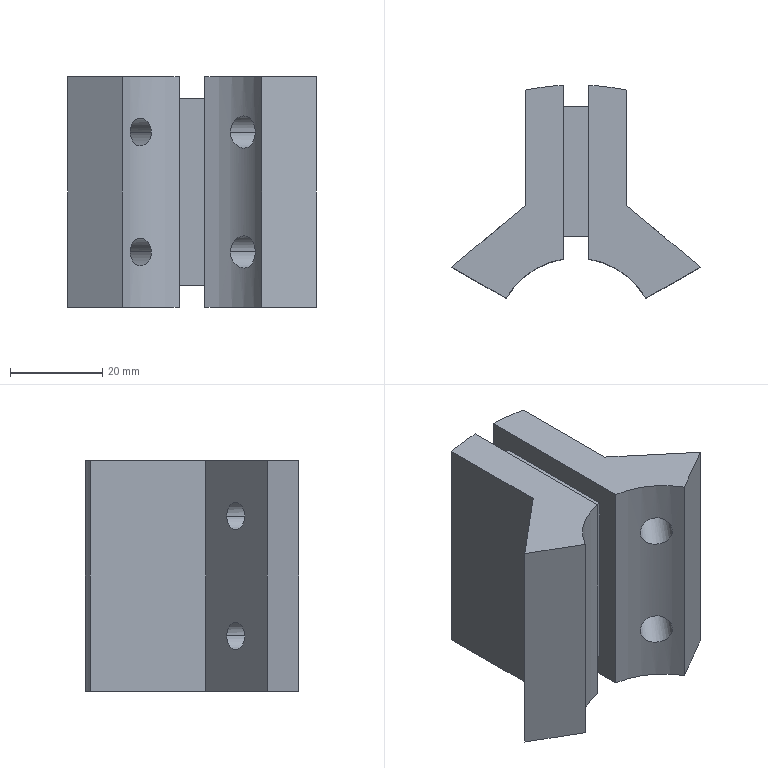Part | SolidWorks | features 3DProfileFeature 2, HoleWzd 2, Extrusion 1, ICE 1 | 1 solid | 28 faces | box 53.823 x 46.181 x 50 mm | volume 52873 mm3 | plane 16 | cylinder 12 | commonest cylinder face diameters 6 x4 7 x4 35 x2 110 x2
STEP:
#1=CARTESIAN_POINT('',(13.703,10.885,13.));
#2=VERTEX_POINT('',#1);
#3=CARTESIAN_POINT('',(8.34,15.385,13.));
#4=VERTEX_POINT('',#3);
#5=CARTESIAN_POINT('',(13.703,10.885,13.));
#6=CARTESIAN_POINT('',(13.703,10.885,12.771));
#7=CARTESIAN_POINT('',(13.689,10.903,12.544));
#8=CARTESIAN_POINT('',(13.631,10.975,12.09));
#9=CARTESIAN_POINT('',(13.588,11.028,11.87));
#10=CARTESIAN_POINT('',(13.476,11.165,11.449));
#11=CARTESIAN_POINT('',(13.405,11.251,11.245));
#12=CARTESIAN_POINT('',(13.237,11.447,10.864));
#13=CARTESIAN_POINT('',(13.141,11.558,10.688));
#14=CARTESIAN_POINT('',(12.924,11.8,10.365));
#15=CARTESIAN_POINT('',(12.801,11.934,10.218));
#16=CARTESIAN_POINT('',(12.538,12.21,9.964));
#17=CARTESIAN_POINT('',(12.397,12.353,9.856));
#18=CARTESIAN_POINT('',(12.093,12.651,9.68));
#19=CARTESIAN_POINT('',(11.932,12.804,9.613));
#20=CARTESIAN_POINT('',(11.6,13.105,9.523));
#21=CARTESIAN_POINT('',(11.427,13.256,9.5));
#22=CARTESIAN_POINT('',(11.073,13.553,9.5));
#23=CARTESIAN_POINT('',(10.896,13.696,9.522));
#24=CARTESIAN_POINT('',(10.541,13.971,9.611));
#25=CARTESIAN_POINT('',(10.362,14.104,9.679));
#26=CARTESIAN_POINT('',(10.017,14.351,9.854));
#27=CARTESIAN_POINT('',(9.85,14.466,9.962));
#28=CARTESIAN_POINT('',(9.531,14.678,10.216));
#29=CARTESIAN_POINT('',(9.379,14.775,10.363));
#30=CARTESIAN_POINT('',(8.965,15.033,10.845));
#31=CARTESIAN_POINT('',(8.735,15.165,11.234));
#32=CARTESIAN_POINT('',(8.502,15.296,11.866));
#33=CARTESIAN_POINT('',(8.442,15.329,12.088));
#34=CARTESIAN_POINT('',(8.361,15.374,12.539));
#35=CARTESIAN_POINT('',(8.34,15.385,12.768));
#36=CARTESIAN_POINT('',(8.34,15.385,13.));
#37=B_SPLINE_CURVE_WITH_KNOTS('',3,(#5,#6,#7,#8,#9,#10,#11,#12,#13,#14,#15,#16,#17,#18,#19,#20,#21,#22,#23,#24,#25,#26,#27,#28,#29,#30,#31,#32,#33,#34,#35,#36),.UNSPECIFIED.,.F.,.F.,(4,2,2,2,2,2,2,2,2,2,2,2,2,2,2,4),(0.01097,0.01166,0.01234,0.01303,0.01371,0.0144,0.01508,0.01577,0.01645,0.01714,0.01782,0.01851,0.0192,0.02057,0.02125,0.02194),.UNSPECIFIED.);
#38=EDGE_CURVE('',#2,#4,#37,.T.);
#39=ORIENTED_EDGE('',*,*,#38,.F.);
#40=CARTESIAN_POINT('',(21.451,20.119,13.));
#41=VERTEX_POINT('',#40);
#42=CARTESIAN_POINT('',(21.451,20.119,13.));
#43=DIRECTION('',(0.6428,0.766,0.));
#44=VECTOR('',#43,1000.);
#45=LINE('',#42,#44);
#46=EDGE_CURVE('',#2,#41,#45,.T.);
#47=ORIENTED_EDGE('',*,*,#46,.T.);
#48=CARTESIAN_POINT('',(16.089,24.619,13.));
#49=VERTEX_POINT('',#48);
#50=CARTESIAN_POINT('',(18.77,22.369,13.));
#51=DIRECTION('',(0.6428,0.766,0.));
#52=DIRECTION('',(-0.766,0.6428,0.));
#53=AXIS2_PLACEMENT_3D('',#50,#51,#52);
#54=CIRCLE('',#53,3.5);
#55=EDGE_CURVE('',#41,#49,#54,.T.);
#56=ORIENTED_EDGE('',*,*,#55,.T.);
#57=CARTESIAN_POINT('',(16.089,24.619,13.));
#58=DIRECTION('',(0.6428,0.766,0.));
#59=VECTOR('',#58,1000.);
#60=LINE('',#57,#59);
#61=EDGE_CURVE('',#4,#49,#60,.T.);
#62=ORIENTED_EDGE('',*,*,#61,.F.);
#63=EDGE_LOOP('',(#39,#47,#56,#62));
#64=FACE_OUTER_BOUND('',#63,.T.);
#65=CARTESIAN_POINT('',(18.77,22.369,13.));
#66=DIRECTION('',(0.6428,0.766,0.));
#67=DIRECTION('',(-0.766,0.6428,0.));
#68=AXIS2_PLACEMENT_3D('',#65,#66,#67);
#69=CYLINDRICAL_SURFACE('',#68,3.5);
#70=ADVANCED_FACE('',(#64),#69,.F.);
#71=CARTESIAN_POINT('',(13.703,10.885,-13.));
#72=VERTEX_POINT('',#71);
#73=CARTESIAN_POINT('',(8.34,15.385,-13.));
#74=VERTEX_POINT('',#73);
#75=CARTESIAN_POINT('',(13.703,10.885,-13.));
#76=CARTESIAN_POINT('',(13.703,10.885,-13.229));
#77=CARTESIAN_POINT('',(13.689,10.903,-13.456));
#78=CARTESIAN_POINT('',(13.631,10.975,-13.91));
#79=CARTESIAN_POINT('',(13.588,11.028,-14.13));
#80=CARTESIAN_POINT('',(13.476,11.165,-14.551));
#81=CARTESIAN_POINT('',(13.405,11.251,-14.755));
#82=CARTESIAN_POINT('',(13.237,11.447,-15.136));
#83=CARTESIAN_POINT('',(13.141,11.558,-15.312));
#84=CARTESIAN_POINT('',(12.924,11.8,-15.635));
#85=CARTESIAN_POINT('',(12.801,11.934,-15.782));
#86=CARTESIAN_POINT('',(12.538,12.21,-16.036));
#87=CARTESIAN_POINT('',(12.397,12.353,-16.144));
#88=CARTESIAN_POINT('',(12.093,12.651,-16.32));
#89=CARTESIAN_POINT('',(11.932,12.804,-16.387));
#90=CARTESIAN_POINT('',(11.6,13.105,-16.477));
#91=CARTESIAN_POINT('',(11.427,13.256,-16.5));
#92=CARTESIAN_POINT('',(11.073,13.553,-16.5));
#93=CARTESIAN_POINT('',(10.896,13.696,-16.478));
#94=CARTESIAN_POINT('',(10.541,13.971,-16.389));
#95=CARTESIAN_POINT('',(10.362,14.104,-16.321));
#96=CARTESIAN_POINT('',(10.017,14.351,-16.146));
#97=CARTESIAN_POINT('',(9.85,14.466,-16.038));
#98=CARTESIAN_POINT('',(9.531,14.678,-15.784));
#99=CARTESIAN_POINT('',(9.379,14.775,-15.637));
#100=CARTESIAN_POINT('',(8.965,15.033,-15.155));
#101=CARTESIAN_POINT('',(8.735,15.165,-14.766));
#102=CARTESIAN_POINT('',(8.502,15.296,-14.134));
#103=CARTESIAN_POINT('',(8.442,15.329,-13.912));
#104=CARTESIAN_POINT('',(8.361,15.374,-13.461));
#105=CARTESIAN_POINT('',(8.34,15.385,-13.232));
#106=CARTESIAN_POINT('',(8.34,15.385,-13.));
#107=B_SPLINE_CURVE_WITH_KNOTS('',3,(#75,#76,#77,#78,#79,#80,#81,#82,#83,#84,#85,#86,#87,#88,#89,#90,#91,#92,#93,#94,#95,#96,#97,#98,#99,#100,#101,#102,#103,#104,#105,#106),.UNSPECIFIED.,.F.,.F.,(4,2,2,2,2,2,2,2,2,2,2,2,2,2,2,4),(0.01097,0.01166,0.01234,0.01303,0.01371,0.0144,0.01508,0.01577,0.01645,0.01714,0.01782,0.01851,0.0192,0.02057,0.02125,0.02194),.UNSPECIFIED.);
#108=EDGE_CURVE('',#72,#74,#107,.T.);
#109=ORIENTED_EDGE('',*,*,#108,.F.);
#110=CARTESIAN_POINT('',(21.451,20.119,-13.));
#111=VERTEX_POINT('',#110);
#112=CARTESIAN_POINT('',(21.451,20.119,-13.));
#113=DIRECTION('',(0.6428,0.766,0.));
#114=VECTOR('',#113,1000.);
#115=LINE('',#112,#114);
#116=EDGE_CURVE('',#72,#111,#115,.T.);
#117=ORIENTED_EDGE('',*,*,#116,.T.);
#118=CARTESIAN_POINT('',(16.089,24.619,-13.));
#119=VERTEX_POINT('',#118);
#120=CARTESIAN_POINT('',(18.77,22.369,-13.));
#121=DIRECTION('',(0.6428,0.766,0.));
#122=DIRECTION('',(-0.766,0.6428,0.));
#123=AXIS2_PLACEMENT_3D('',#120,#121,#122);
#124=CIRCLE('',#123,3.5);
#125=EDGE_CURVE('',#111,#119,#124,.T.);
#126=ORIENTED_EDGE('',*,*,#125,.T.);
#127=CARTESIAN_POINT('',(16.089,24.619,-13.));
#128=DIRECTION('',(0.6428,0.766,0.));
#129=VECTOR('',#128,1000.);
#130=LINE('',#127,#129);
#131=EDGE_CURVE('',#74,#119,#130,.T.);
#132=ORIENTED_EDGE('',*,*,#131,.F.);
#133=EDGE_LOOP('',(#109,#117,#126,#132));
#134=FACE_OUTER_BOUND('',#133,.T.);
#135=CARTESIAN_POINT('',(18.77,22.369,-13.));
#136=DIRECTION('',(0.6428,0.766,0.));
#137=DIRECTION('',(-0.766,0.6428,0.));
#138=AXIS2_PLACEMENT_3D('',#135,#136,#137);
#139=CYLINDRICAL_SURFACE('',#138,3.5);
#140=ADVANCED_FACE('',(#134),#139,.F.);
#141=CARTESIAN_POINT('',(-8.784,15.136,-13.));
#142=VERTEX_POINT('',#141);
#143=CARTESIAN_POINT('',(-13.38,11.279,-13.));
#144=VERTEX_POINT('',#143);
#145=CARTESIAN_POINT('',(-8.784,15.136,-13.));
#146=CARTESIAN_POINT('',(-8.784,15.136,-13.196));
#147=CARTESIAN_POINT('',(-8.801,15.126,-13.391));
#148=CARTESIAN_POINT('',(-8.868,15.087,-13.779));
#149=CARTESIAN_POINT('',(-8.919,15.057,-13.968));
#150=CARTESIAN_POINT('',(-9.049,14.979,-14.329));
#151=CARTESIAN_POINT('',(-9.13,14.93,-14.504));
#152=CARTESIAN_POINT('',(-9.317,14.814,-14.831));
#153=CARTESIAN_POINT('',(-9.423,14.747,-14.982));
#154=CARTESIAN_POINT('',(-9.656,14.595,-15.258));
#155=CARTESIAN_POINT('',(-9.785,14.509,-15.385));
#156=CARTESIAN_POINT('',(-10.054,14.324,-15.602));
#157=CARTESIAN_POINT('',(-10.195,14.225,-15.695));
#158=CARTESIAN_POINT('',(-10.489,14.009,-15.846));
#159=CARTESIAN_POINT('',(-10.641,13.894,-15.904));
#160=CARTESIAN_POINT('',(-10.943,13.658,-15.98));
#161=CARTESIAN_POINT('',(-11.096,13.534,-16.));
#162=CARTESIAN_POINT('',(-11.399,13.28,-16.));
#163=CARTESIAN_POINT('',(-11.547,13.152,-15.981));
#164=CARTESIAN_POINT('',(-11.833,12.895,-15.905));
#165=CARTESIAN_POINT('',(-11.973,12.765,-15.847));
#166=CARTESIAN_POINT('',(-12.235,12.513,-15.697));
#167=CARTESIAN_POINT('',(-12.358,12.392,-15.605));
#168=CARTESIAN_POINT('',(-12.588,12.158,-15.387));
#169=CARTESIAN_POINT('',(-12.695,12.046,-15.261));
#170=CARTESIAN_POINT('',(-12.98,11.741,-14.847));
#171=CARTESIAN_POINT('',(-13.129,11.571,-14.513));
#172=CARTESIAN_POINT('',(-13.279,11.399,-13.972));
#173=CARTESIAN_POINT('',(-13.317,11.354,-13.782));
#174=CARTESIAN_POINT('',(-13.368,11.294,-13.395));
#175=CARTESIAN_POINT('',(-13.38,11.279,-13.199));
#176=CARTESIAN_POINT('',(-13.38,11.279,-13.));
#177=B_SPLINE_CURVE_WITH_KNOTS('',3,(#145,#146,#147,#148,#149,#150,#151,#152,#153,#154,#155,#156,#157,#158,#159,#160,#161,#162,#163,#164,#165,#166,#167,#168,#169,#170,#171,#172,#173,#174,#175,#176),.UNSPECIFIED.,.F.,.F.,(4,2,2,2,2,2,2,2,2,2,2,2,2,2,2,4),(0.009397,0.009984,0.01057,0.01116,0.01175,0.01233,0.01292,0.01351,0.01409,0.01468,0.01527,0.01586,0.01644,0.01762,0.0182,0.01879),.UNSPECIFIED.);
#178=EDGE_CURVE('',#142,#144,#177,.T.);
#179=ORIENTED_EDGE('',*,*,#178,.F.);
#180=CARTESIAN_POINT('',(-16.472,24.297,-13.));
#181=VERTEX_POINT('',#180);
#182=CARTESIAN_POINT('',(-16.472,24.297,-13.));
#183=DIRECTION('',(-0.6428,0.766,0.));
#184=VECTOR('',#183,1000.);
#185=LINE('',#182,#184);
#186=EDGE_CURVE('',#142,#181,#185,.T.);
#187=ORIENTED_EDGE('',*,*,#186,.T.);
#188=CARTESIAN_POINT('',(-21.068,20.441,-13.));
#189=VERTEX_POINT('',#188);
#190=CARTESIAN_POINT('',(-18.77,22.369,-13.));
#191=DIRECTION('',(-0.6428,0.766,0.));
#192=DIRECTION('',(-0.766,-0.6428,0.));
#193=AXIS2_PLACEMENT_3D('',#190,#191,#192);
#194=CIRCLE('',#193,3.);
#195=EDGE_CURVE('',#181,#189,#194,.T.);
#196=ORIENTED_EDGE('',*,*,#195,.T.);
#197=CARTESIAN_POINT('',(-21.068,20.441,-13.));
#198=DIRECTION('',(-0.6428,0.766,0.));
#199=VECTOR('',#198,1000.);
#200=LINE('',#197,#199);
#201=EDGE_CURVE('',#144,#189,#200,.T.);
#202=ORIENTED_EDGE('',*,*,#201,.F.);
#203=EDGE_LOOP('',(#179,#187,#196,#202));
#204=FACE_OUTER_BOUND('',#203,.T.);
#205=CARTESIAN_POINT('',(-18.77,22.369,-13.));
#206=DIRECTION('',(-0.6428,0.766,0.));
#207=DIRECTION('',(-0.766,-0.6428,0.));
#208=AXIS2_PLACEMENT_3D('',#205,#206,#207);
#209=CYLINDRICAL_SURFACE('',#208,3.);
#210=ADVANCED_FACE('',(#204),#209,.F.);
#211=CARTESIAN_POINT('',(-8.784,15.136,13.));
#212=VERTEX_POINT('',#211);
#213=CARTESIAN_POINT('',(-13.38,11.279,13.));
#214=VERTEX_POINT('',#213);
#215=CARTESIAN_POINT('',(-8.784,15.136,13.));
#216=CARTESIAN_POINT('',(-8.784,15.136,12.804));
#217=CARTESIAN_POINT('',(-8.801,15.126,12.609));
#218=CARTESIAN_POINT('',(-8.868,15.087,12.221));
#219=CARTESIAN_POINT('',(-8.919,15.057,12.032));
#220=CARTESIAN_POINT('',(-9.049,14.979,11.671));
#221=CARTESIAN_POINT('',(-9.13,14.93,11.496));
#222=CARTESIAN_POINT('',(-9.317,14.814,11.169));
#223=CARTESIAN_POINT('',(-9.423,14.747,11.018));
#224=CARTESIAN_POINT('',(-9.656,14.595,10.742));
#225=CARTESIAN_POINT('',(-9.785,14.509,10.615));
#226=CARTESIAN_POINT('',(-10.054,14.324,10.398));
#227=CARTESIAN_POINT('',(-10.195,14.225,10.305));
#228=CARTESIAN_POINT('',(-10.489,14.009,10.154));
#229=CARTESIAN_POINT('',(-10.641,13.894,10.096));
#230=CARTESIAN_POINT('',(-10.943,13.658,10.02));
#231=CARTESIAN_POINT('',(-11.096,13.534,10.));
#232=CARTESIAN_POINT('',(-11.399,13.28,10.));
#233=CARTESIAN_POINT('',(-11.547,13.152,10.019));
#234=CARTESIAN_POINT('',(-11.833,12.895,10.095));
#235=CARTESIAN_POINT('',(-11.973,12.765,10.153));
#236=CARTESIAN_POINT('',(-12.235,12.513,10.303));
#237=CARTESIAN_POINT('',(-12.358,12.392,10.395));
#238=CARTESIAN_POINT('',(-12.588,12.158,10.613));
#239=CARTESIAN_POINT('',(-12.695,12.046,10.739));
#240=CARTESIAN_POINT('',(-12.98,11.741,11.153));
#241=CARTESIAN_POINT('',(-13.129,11.571,11.487));
#242=CARTESIAN_POINT('',(-13.279,11.399,12.028));
#243=CARTESIAN_POINT('',(-13.317,11.354,12.218));
#244=CARTESIAN_POINT('',(-13.368,11.294,12.605));
#245=CARTESIAN_POINT('',(-13.38,11.279,12.801));
#246=CARTESIAN_POINT('',(-13.38,11.279,13.));
#247=B_SPLINE_CURVE_WITH_KNOTS('',3,(#215,#216,#217,#218,#219,#220,#221,#222,#223,#224,#225,#226,#227,#228,#229,#230,#231,#232,#233,#234,#235,#236,#237,#238,#239,#240,#241,#242,#243,#244,#245,#246),.UNSPECIFIED.,.F.,.F.,(4,2,2,2,2,2,2,2,2,2,2,2,2,2,2,4),(0.009397,0.009984,0.01057,0.01116,0.01175,0.01233,0.01292,0.01351,0.01409,0.01468,0.01527,0.01586,0.01644,0.01762,0.0182,0.01879),.UNSPECIFIED.);
#248=EDGE_CURVE('',#212,#214,#247,.T.);
#249=ORIENTED_EDGE('',*,*,#248,.F.);
#250=CARTESIAN_POINT('',(-16.472,24.297,13.));
#251=VERTEX_POINT('',#250);
#252=CARTESIAN_POINT('',(-16.472,24.297,13.));
#253=DIRECTION('',(-0.6428,0.766,0.));
#254=VECTOR('',#253,1000.);
#255=LINE('',#252,#254);
#256=EDGE_CURVE('',#212,#251,#255,.T.);
#257=ORIENTED_EDGE('',*,*,#256,.T.);
#258=CARTESIAN_POINT('',(-21.068,20.441,13.));
#259=VERTEX_POINT('',#258);
#260=CARTESIAN_POINT('',(-18.77,22.369,13.));
#261=DIRECTION('',(-0.6428,0.766,0.));
#262=DIRECTION('',(-0.766,-0.6428,0.));
#263=AXIS2_PLACEMENT_3D('',#260,#261,#262);
#264=CIRCLE('',#263,3.);
#265=EDGE_CURVE('',#251,#259,#264,.T.);
#266=ORIENTED_EDGE('',*,*,#265,.T.);
#267=CARTESIAN_POINT('',(-21.068,20.441,13.));
#268=DIRECTION('',(-0.6428,0.766,0.));
#269=VECTOR('',#268,1000.);
#270=LINE('',#267,#269);
#271=EDGE_CURVE('',#214,#259,#270,.T.);
#272=ORIENTED_EDGE('',*,*,#271,.F.);
#273=EDGE_LOOP('',(#249,#257,#266,#272));
#274=FACE_OUTER_BOUND('',#273,.T.);
#275=CARTESIAN_POINT('',(-18.77,22.369,13.));
#276=DIRECTION('',(-0.6428,0.766,0.));
#277=DIRECTION('',(-0.766,-0.6428,0.));
#278=AXIS2_PLACEMENT_3D('',#275,#276,#277);
#279=CYLINDRICAL_SURFACE('',#278,3.);
#280=ADVANCED_FACE('',(#274),#279,.F.);
#281=CARTESIAN_POINT('',(-2.75,54.931,-25.));
#282=VERTEX_POINT('',#281);
#283=CARTESIAN_POINT('',(-11.,53.889,-25.));
#284=VERTEX_POINT('',#283);
#285=CARTESIAN_POINT('',(0.,0.,-25.));
#286=DIRECTION('',(0.,0.,1.));
#287=DIRECTION('',(1.,0.,0.));
#288=AXIS2_PLACEMENT_3D('',#285,#286,#287);
#289=CIRCLE('',#288,55.);
#290=EDGE_CURVE('',#282,#284,#289,.T.);
#291=ORIENTED_EDGE('',*,*,#290,.T.);
#292=CARTESIAN_POINT('',(-11.,53.889,25.));
#293=VERTEX_POINT('',#292);
#294=CARTESIAN_POINT('',(-11.,53.889,25.));
#295=DIRECTION('',(0.,0.,-1.));
#296=VECTOR('',#295,1000.);
#297=LINE('',#294,#296);
#298=EDGE_CURVE('',#293,#284,#297,.T.);
#299=ORIENTED_EDGE('',*,*,#298,.F.);
#300=CARTESIAN_POINT('',(-2.75,54.931,25.));
#301=VERTEX_POINT('',#300);
#302=CARTESIAN_POINT('',(0.,0.,25.));
#303=DIRECTION('',(0.,0.,1.));
#304=DIRECTION('',(1.,0.,0.));
#305=AXIS2_PLACEMENT_3D('',#302,#303,#304);
#306=CIRCLE('',#305,55.);
#307=EDGE_CURVE('',#301,#293,#306,.T.);
#308=ORIENTED_EDGE('',*,*,#307,.F.);
#309=CARTESIAN_POINT('',(-2.75,54.931,25.));
#310=DIRECTION('',(0.,0.,-1.));
#311=VECTOR('',#310,1000.);
#312=LINE('',#309,#311);
#313=EDGE_CURVE('',#301,#282,#312,.T.);
#314=ORIENTED_EDGE('',*,*,#313,.T.);
#315=EDGE_LOOP('',(#291,#299,#308,#314));
#316=FACE_OUTER_BOUND('',#315,.T.);
#317=CARTESIAN_POINT('',(0.,0.,25.));
#318=DIRECTION('',(0.,0.,-1.));
#319=DIRECTION('',(-1.,0.,0.));
#320=AXIS2_PLACEMENT_3D('',#317,#318,#319);
#321=CYLINDRICAL_SURFACE('',#320,55.);
#322=ADVANCED_FACE('',(#316),#321,.T.);
#323=CARTESIAN_POINT('',(-11.,28.889,-25.));
#324=VERTEX_POINT('',#323);
#325=CARTESIAN_POINT('',(-11.,53.889,-25.));
#326=DIRECTION('',(0.,-1.,0.));
#327=VECTOR('',#326,1000.);
#328=LINE('',#325,#327);
#329=EDGE_CURVE('',#284,#324,#328,.T.);
#330=ORIENTED_EDGE('',*,*,#329,.T.);
#331=CARTESIAN_POINT('',(-11.,28.889,25.));
#332=VERTEX_POINT('',#331);
#333=CARTESIAN_POINT('',(-11.,28.889,25.));
#334=DIRECTION('',(0.,0.,-1.));
#335=VECTOR('',#334,1000.);
#336=LINE('',#333,#335);
#337=EDGE_CURVE('',#332,#324,#336,.T.);
#338=ORIENTED_EDGE('',*,*,#337,.F.);
#339=CARTESIAN_POINT('',(-11.,53.889,25.));
#340=DIRECTION('',(0.,-1.,0.));
#341=VECTOR('',#340,1000.);
#342=LINE('',#339,#341);
#343=EDGE_CURVE('',#293,#332,#342,.T.);
#344=ORIENTED_EDGE('',*,*,#343,.F.);
#345=ORIENTED_EDGE('',*,*,#298,.T.);
#346=EDGE_LOOP('',(#330,#338,#344,#345));
#347=FACE_OUTER_BOUND('',#346,.T.);
#348=CARTESIAN_POINT('',(-11.,53.889,25.));
#349=DIRECTION('',(1.,0.,0.));
#350=DIRECTION('',(0.,1.,0.));
#351=AXIS2_PLACEMENT_3D('',#348,#349,#350);
#352=PLANE('',#351);
#353=ADVANCED_FACE('',(#347),#352,.F.);
#354=CARTESIAN_POINT('',(-18.77,22.369,-13.));
#355=DIRECTION('',(-0.6428,0.766,0.));
#356=DIRECTION('',(-0.766,-0.6428,0.));
#357=AXIS2_PLACEMENT_3D('',#354,#355,#356);
#358=CIRCLE('',#357,3.);
#359=EDGE_CURVE('',#189,#181,#358,.T.);
#360=ORIENTED_EDGE('',*,*,#359,.F.);
#361=ORIENTED_EDGE('',*,*,#195,.F.);
#362=EDGE_LOOP('',(#360,#361));
#363=FACE_BOUND('',#362,.T.);
#364=CARTESIAN_POINT('',(-18.77,22.369,13.));
#365=DIRECTION('',(-0.6428,0.766,0.));
#366=DIRECTION('',(-0.766,-0.6428,0.));
#367=AXIS2_PLACEMENT_3D('',#364,#365,#366);
#368=CIRCLE('',#367,3.);
#369=EDGE_CURVE('',#259,#251,#368,.T.);
#370=ORIENTED_EDGE('',*,*,#369,.F.);
#371=ORIENTED_EDGE('',*,*,#265,.F.);
#372=EDGE_LOOP('',(#370,#371));
#373=FACE_BOUND('',#372,.T.);
#374=CARTESIAN_POINT('',(-26.912,15.537,-25.));
#375=VERTEX_POINT('',#374);
#376=CARTESIAN_POINT('',(-11.,28.889,-25.));
#377=DIRECTION('',(-0.766,-0.6428,0.));
#378=VECTOR('',#377,1000.);
#379=LINE('',#376,#378);
#380=EDGE_CURVE('',#324,#375,#379,.T.);
#381=ORIENTED_EDGE('',*,*,#380,.T.);
#382=CARTESIAN_POINT('',(-26.912,15.537,25.));
#383=VERTEX_POINT('',#382);
#384=CARTESIAN_POINT('',(-26.912,15.537,25.));
#385=DIRECTION('',(0.,0.,-1.));
#386=VECTOR('',#385,1000.);
#387=LINE('',#384,#386);
#388=EDGE_CURVE('',#383,#375,#387,.T.);
#389=ORIENTED_EDGE('',*,*,#388,.F.);
#390=CARTESIAN_POINT('',(-11.,28.889,25.));
#391=DIRECTION('',(-0.766,-0.6428,0.));
#392=VECTOR('',#391,1000.);
#393=LINE('',#390,#392);
#394=EDGE_CURVE('',#332,#383,#393,.T.);
#395=ORIENTED_EDGE('',*,*,#394,.F.);
#396=ORIENTED_EDGE('',*,*,#337,.T.);
#397=EDGE_LOOP('',(#381,#389,#395,#396));
#398=FACE_OUTER_BOUND('',#397,.T.);
#399=CARTESIAN_POINT('',(-11.,28.889,25.));
#400=DIRECTION('',(0.6428,-0.766,0.));
#401=DIRECTION('',(0.766,0.6428,0.));
#402=AXIS2_PLACEMENT_3D('',#399,#400,#401);
#403=PLANE('',#402);
#404=ADVANCED_FACE('',(#363,#373,#398),#403,.F.);
#405=CARTESIAN_POINT('',(-15.155,8.75,-25.));
#406=VERTEX_POINT('',#405);
#407=CARTESIAN_POINT('',(-26.912,15.537,-25.));
#408=DIRECTION('',(0.866,-0.5,0.));
#409=VECTOR('',#408,1000.);
#410=LINE('',#407,#409);
#411=EDGE_CURVE('',#375,#406,#410,.T.);
#412=ORIENTED_EDGE('',*,*,#411,.T.);
#413=CARTESIAN_POINT('',(-15.155,8.75,25.));
#414=VERTEX_POINT('',#413);
#415=CARTESIAN_POINT('',(-15.155,8.75,25.));
#416=DIRECTION('',(0.,0.,-1.));
#417=VECTOR('',#416,1000.);
#418=LINE('',#415,#417);
#419=EDGE_CURVE('',#414,#406,#418,.T.);
#420=ORIENTED_EDGE('',*,*,#419,.F.);
#421=CARTESIAN_POINT('',(-26.912,15.537,25.));
#422=DIRECTION('',(0.866,-0.5,0.));
#423=VECTOR('',#422,1000.);
#424=LINE('',#421,#423);
#425=EDGE_CURVE('',#383,#414,#424,.T.);
#426=ORIENTED_EDGE('',*,*,#425,.F.);
#427=ORIENTED_EDGE('',*,*,#388,.T.);
#428=EDGE_LOOP('',(#412,#420,#426,#427));
#429=FACE_OUTER_BOUND('',#428,.T.);
#430=CARTESIAN_POINT('',(-26.912,15.537,25.));
#431=DIRECTION('',(0.5,0.866,0.));
#432=DIRECTION('',(-0.866,0.5,0.));
#433=AXIS2_PLACEMENT_3D('',#430,#431,#432);
#434=PLANE('',#433);
#435=ADVANCED_FACE('',(#429),#434,.F.);
#436=CARTESIAN_POINT('',(-13.38,11.279,-13.));
#437=CARTESIAN_POINT('',(-13.38,11.279,-12.801));
#438=CARTESIAN_POINT('',(-13.368,11.294,-12.606));
#439=CARTESIAN_POINT('',(-13.317,11.353,-12.222));
#440=CARTESIAN_POINT('',(-13.279,11.398,-12.031));
#441=CARTESIAN_POINT('',(-13.179,11.513,-11.668));
#442=CARTESIAN_POINT('',(-13.118,11.584,-11.496));
#443=CARTESIAN_POINT('',(-12.971,11.748,-11.17));
#444=CARTESIAN_POINT('',(-12.886,11.842,-11.016));
#445=CARTESIAN_POINT('',(-12.696,12.045,-10.74));
#446=CARTESIAN_POINT('',(-12.591,12.155,-10.616));
#447=CARTESIAN_POINT('',(-12.36,12.39,-10.397));
#448=CARTESIAN_POINT('',(-12.236,12.513,-10.304));
#449=CARTESIAN_POINT('',(-11.974,12.763,-10.154));
#450=CARTESIAN_POINT('',(-11.836,12.892,-10.096));
#451=CARTESIAN_POINT('',(-11.547,13.151,-10.019));
#452=CARTESIAN_POINT('',(-11.4,13.279,-10.));
#453=CARTESIAN_POINT('',(-11.099,13.531,-10.));
#454=CARTESIAN_POINT('',(-10.945,13.657,-10.02));
#455=CARTESIAN_POINT('',(-10.641,13.894,-10.096));
#456=CARTESIAN_POINT('',(-10.492,14.007,-10.153));
#457=CARTESIAN_POINT('',(-10.198,14.223,-10.304));
#458=CARTESIAN_POINT('',(-10.055,14.324,-10.398));
#459=CARTESIAN_POINT('',(-9.786,14.509,-10.615));
#460=CARTESIAN_POINT('',(-9.659,14.594,-10.739));
#461=CARTESIAN_POINT('',(-9.423,14.747,-11.018));
#462=CARTESIAN_POINT('',(-9.317,14.814,-11.17));
#463=CARTESIAN_POINT('',(-9.131,14.93,-11.494));
#464=CARTESIAN_POINT('',(-9.049,14.979,-11.67));
#465=CARTESIAN_POINT('',(-8.919,15.057,-12.033));
#466=CARTESIAN_POINT('',(-8.869,15.086,-12.22));
#467=CARTESIAN_POINT('',(-8.801,15.126,-12.605));
#468=CARTESIAN_POINT('',(-8.784,15.136,-12.804));
#469=CARTESIAN_POINT('',(-8.784,15.136,-13.));
#470=B_SPLINE_CURVE_WITH_KNOTS('',3,(#436,#437,#438,#439,#440,#441,#442,#443,#444,#445,#446,#447,#448,#449,#450,#451,#452,#453,#454,#455,#456,#457,#458,#459,#460,#461,#462,#463,#464,#465,#466,#467,#468,#469),.UNSPECIFIED.,.F.,.F.,(4,2,2,2,2,2,2,2,2,2,2,2,2,2,2,2,4),(0.,0.0005873,0.001175,0.001762,0.002349,0.002936,0.003524,0.004111,0.004698,0.005286,0.005873,0.00646,0.007048,0.007635,0.008222,0.008809,0.009397),.UNSPECIFIED.);
#471=EDGE_CURVE('',#144,#142,#470,.T.);
#472=ORIENTED_EDGE('',*,*,#471,.T.);
#473=ORIENTED_EDGE('',*,*,#178,.T.);
#474=EDGE_LOOP('',(#472,#473));
#475=FACE_BOUND('',#474,.T.);
#476=CARTESIAN_POINT('',(-13.38,11.279,13.));
#477=CARTESIAN_POINT('',(-13.38,11.279,13.199));
#478=CARTESIAN_POINT('',(-13.368,11.294,13.394));
#479=CARTESIAN_POINT('',(-13.317,11.353,13.778));
#480=CARTESIAN_POINT('',(-13.279,11.398,13.969));
#481=CARTESIAN_POINT('',(-13.179,11.513,14.332));
#482=CARTESIAN_POINT('',(-13.118,11.584,14.504));
#483=CARTESIAN_POINT('',(-12.971,11.748,14.83));
#484=CARTESIAN_POINT('',(-12.886,11.842,14.984));
#485=CARTESIAN_POINT('',(-12.696,12.045,15.26));
#486=CARTESIAN_POINT('',(-12.591,12.155,15.384));
#487=CARTESIAN_POINT('',(-12.36,12.39,15.603));
#488=CARTESIAN_POINT('',(-12.236,12.513,15.696));
#489=CARTESIAN_POINT('',(-11.974,12.763,15.846));
#490=CARTESIAN_POINT('',(-11.836,12.892,15.904));
#491=CARTESIAN_POINT('',(-11.547,13.151,15.981));
#492=CARTESIAN_POINT('',(-11.4,13.279,16.));
#493=CARTESIAN_POINT('',(-11.099,13.531,16.));
#494=CARTESIAN_POINT('',(-10.945,13.657,15.98));
#495=CARTESIAN_POINT('',(-10.641,13.894,15.904));
#496=CARTESIAN_POINT('',(-10.492,14.007,15.847));
#497=CARTESIAN_POINT('',(-10.198,14.223,15.696));
#498=CARTESIAN_POINT('',(-10.055,14.324,15.602));
#499=CARTESIAN_POINT('',(-9.786,14.509,15.385));
#500=CARTESIAN_POINT('',(-9.659,14.594,15.261));
#501=CARTESIAN_POINT('',(-9.423,14.747,14.982));
#502=CARTESIAN_POINT('',(-9.317,14.814,14.83));
#503=CARTESIAN_POINT('',(-9.131,14.93,14.506));
#504=CARTESIAN_POINT('',(-9.049,14.979,14.33));
#505=CARTESIAN_POINT('',(-8.919,15.057,13.967));
#506=CARTESIAN_POINT('',(-8.869,15.086,13.78));
#507=CARTESIAN_POINT('',(-8.801,15.126,13.395));
#508=CARTESIAN_POINT('',(-8.784,15.136,13.196));
#509=CARTESIAN_POINT('',(-8.784,15.136,13.));
#510=B_SPLINE_CURVE_WITH_KNOTS('',3,(#476,#477,#478,#479,#480,#481,#482,#483,#484,#485,#486,#487,#488,#489,#490,#491,#492,#493,#494,#495,#496,#497,#498,#499,#500,#501,#502,#503,#504,#505,#506,#507,#508,#509),.UNSPECIFIED.,.F.,.F.,(4,2,2,2,2,2,2,2,2,2,2,2,2,2,2,2,4),(0.,0.0005873,0.001175,0.001762,0.002349,0.002936,0.003524,0.004111,0.004698,0.005286,0.005873,0.00646,0.007048,0.007635,0.008222,0.008809,0.009397),.UNSPECIFIED.);
#511=EDGE_CURVE('',#214,#212,#510,.T.);
#512=ORIENTED_EDGE('',*,*,#511,.T.);
#513=ORIENTED_EDGE('',*,*,#248,.T.);
#514=EDGE_LOOP('',(#512,#513));
#515=FACE_BOUND('',#514,.T.);
#516=CARTESIAN_POINT('',(-2.75,17.283,-25.));
#517=VERTEX_POINT('',#516);
#518=CARTESIAN_POINT('',(0.,0.,-25.));
#519=DIRECTION('',(0.,0.,-1.));
#520=DIRECTION('',(1.,0.,0.));
#521=AXIS2_PLACEMENT_3D('',#518,#519,#520);
#522=CIRCLE('',#521,17.5);
#523=EDGE_CURVE('',#406,#517,#522,.T.);
#524=ORIENTED_EDGE('',*,*,#523,.T.);
#525=CARTESIAN_POINT('',(-2.75,17.283,25.));
#526=VERTEX_POINT('',#525);
#527=CARTESIAN_POINT('',(-2.75,17.283,25.));
#528=DIRECTION('',(0.,0.,-1.));
#529=VECTOR('',#528,1000.);
#530=LINE('',#527,#529);
#531=EDGE_CURVE('',#526,#517,#530,.T.);
#532=ORIENTED_EDGE('',*,*,#531,.F.);
#533=CARTESIAN_POINT('',(0.,0.,25.));
#534=DIRECTION('',(0.,0.,-1.));
#535=DIRECTION('',(1.,0.,0.));
#536=AXIS2_PLACEMENT_3D('',#533,#534,#535);
#537=CIRCLE('',#536,17.5);
#538=EDGE_CURVE('',#414,#526,#537,.T.);
#539=ORIENTED_EDGE('',*,*,#538,.F.);
#540=ORIENTED_EDGE('',*,*,#419,.T.);
#541=EDGE_LOOP('',(#524,#532,#539,#540));
#542=FACE_OUTER_BOUND('',#541,.T.);
#543=CARTESIAN_POINT('',(0.,0.,25.));
#544=DIRECTION('',(0.,0.,-1.));
#545=DIRECTION('',(-1.,0.,0.));
#546=AXIS2_PLACEMENT_3D('',#543,#544,#545);
#547=CYLINDRICAL_SURFACE('',#546,17.5);
#548=ADVANCED_FACE('',(#475,#515,#542),#547,.F.);
#549=CARTESIAN_POINT('',(-2.75,50.3,20.3));
#550=VERTEX_POINT('',#549);
#551=CARTESIAN_POINT('',(-2.75,50.3,-20.3));
#552=VERTEX_POINT('',#551);
#553=CARTESIAN_POINT('',(-2.75,50.3,20.3));
#554=DIRECTION('',(0.,0.,-1.));
#555=VECTOR('',#554,1000.);
#556=LINE('',#553,#555);
#557=EDGE_CURVE('',#550,#552,#556,.T.);
#558=ORIENTED_EDGE('',*,*,#557,.T.);
#559=CARTESIAN_POINT('',(-2.75,22.2,-20.3));
#560=VERTEX_POINT('',#559);
#561=CARTESIAN_POINT('',(-2.75,22.2,-20.3));
#562=DIRECTION('',(0.,-1.,0.));
#563=VECTOR('',#562,1000.);
#564=LINE('',#561,#563);
#565=EDGE_CURVE('',#552,#560,#564,.T.);
#566=ORIENTED_EDGE('',*,*,#565,.T.);
#567=CARTESIAN_POINT('',(-2.75,22.2,20.3));
#568=VERTEX_POINT('',#567);
#569=CARTESIAN_POINT('',(-2.75,22.2,20.3));
#570=DIRECTION('',(0.,0.,-1.));
#571=VECTOR('',#570,1000.);
#572=LINE('',#569,#571);
#573=EDGE_CURVE('',#568,#560,#572,.T.);
#574=ORIENTED_EDGE('',*,*,#573,.F.);
#575=CARTESIAN_POINT('',(-2.75,22.2,20.3));
#576=DIRECTION('',(0.,-1.,0.));
#577=VECTOR('',#576,1000.);
#578=LINE('',#575,#577);
#579=EDGE_CURVE('',#550,#568,#578,.T.);
#580=ORIENTED_EDGE('',*,*,#579,.F.);
#581=EDGE_LOOP('',(#558,#566,#574,#580));
#582=FACE_BOUND('',#581,.T.);
#583=CARTESIAN_POINT('',(-2.75,54.931,-25.));
#584=DIRECTION('',(0.,1.,0.));
#585=VECTOR('',#584,1000.);
#586=LINE('',#583,#585);
#587=EDGE_CURVE('',#517,#282,#586,.T.);
#588=ORIENTED_EDGE('',*,*,#587,.T.);
#589=ORIENTED_EDGE('',*,*,#313,.F.);
#590=CARTESIAN_POINT('',(-2.75,54.931,25.));
#591=DIRECTION('',(0.,1.,0.));
#592=VECTOR('',#591,1000.);
#593=LINE('',#590,#592);
#594=EDGE_CURVE('',#526,#301,#593,.T.);
#595=ORIENTED_EDGE('',*,*,#594,.F.);
#596=ORIENTED_EDGE('',*,*,#531,.T.);
#597=EDGE_LOOP('',(#588,#589,#595,#596));
#598=FACE_OUTER_BOUND('',#597,.T.);
#599=CARTESIAN_POINT('',(-2.75,54.931,25.));
#600=DIRECTION('',(-1.,0.,0.));
#601=DIRECTION('',(0.,-1.,0.));
#602=AXIS2_PLACEMENT_3D('',#599,#600,#601);
#603=PLANE('',#602);
#604=ADVANCED_FACE('',(#582,#598),#603,.F.);
#605=ORIENTED_EDGE('',*,*,#307,.T.);
#606=ORIENTED_EDGE('',*,*,#343,.T.);
#607=ORIENTED_EDGE('',*,*,#394,.T.);
#608=ORIENTED_EDGE('',*,*,#425,.T.);
#609=ORIENTED_EDGE('',*,*,#538,.T.);
#610=ORIENTED_EDGE('',*,*,#594,.T.);
#611=EDGE_LOOP('',(#605,#606,#607,#608,#609,#610));
#612=FACE_OUTER_BOUND('',#611,.T.);
#613=CARTESIAN_POINT('',(0.,0.,25.));
#614=DIRECTION('',(0.,0.,1.));
#615=DIRECTION('',(1.,0.,0.));
#616=AXIS2_PLACEMENT_3D('',#613,#614,#615);
#617=PLANE('',#616);
#618=ADVANCED_FACE('',(#612),#617,.T.);
#619=ORIENTED_EDGE('',*,*,#290,.F.);
#620=ORIENTED_EDGE('',*,*,#587,.F.);
#621=ORIENTED_EDGE('',*,*,#523,.F.);
#622=ORIENTED_EDGE('',*,*,#411,.F.);
#623=ORIENTED_EDGE('',*,*,#380,.F.);
#624=ORIENTED_EDGE('',*,*,#329,.F.);
#625=EDGE_LOOP('',(#619,#620,#621,#622,#623,#624));
#626=FACE_OUTER_BOUND('',#625,.T.);
#627=CARTESIAN_POINT('',(0.,0.,-25.));
#628=DIRECTION('',(0.,0.,1.));
#629=DIRECTION('',(1.,0.,0.));
#630=AXIS2_PLACEMENT_3D('',#627,#628,#629);
#631=PLANE('',#630);
#632=ADVANCED_FACE('',(#626),#631,.F.);
#633=CARTESIAN_POINT('',(2.75,22.2,-20.3));
#634=VERTEX_POINT('',#633);
#635=CARTESIAN_POINT('',(2.75,22.2,-20.3));
#636=DIRECTION('',(1.,0.,0.));
#637=VECTOR('',#636,1000.);
#638=LINE('',#635,#637);
#639=EDGE_CURVE('',#560,#634,#638,.T.);
#640=ORIENTED_EDGE('',*,*,#639,.T.);
#641=CARTESIAN_POINT('',(2.75,22.2,20.3));
#642=VERTEX_POINT('',#641);
#643=CARTESIAN_POINT('',(2.75,22.2,20.3));
#644=DIRECTION('',(0.,0.,-1.));
#645=VECTOR('',#644,1000.);
#646=LINE('',#643,#645);
#647=EDGE_CURVE('',#642,#634,#646,.T.);
#648=ORIENTED_EDGE('',*,*,#647,.F.);
#649=CARTESIAN_POINT('',(2.75,22.2,20.3));
#650=DIRECTION('',(1.,0.,0.));
#651=VECTOR('',#650,1000.);
#652=LINE('',#649,#651);
#653=EDGE_CURVE('',#568,#642,#652,.T.);
#654=ORIENTED_EDGE('',*,*,#653,.F.);
#655=ORIENTED_EDGE('',*,*,#573,.T.);
#656=EDGE_LOOP('',(#640,#648,#654,#655));
#657=FACE_OUTER_BOUND('',#656,.T.);
#658=CARTESIAN_POINT('',(2.75,22.2,20.3));
#659=DIRECTION('',(0.,1.,0.));
#660=DIRECTION('',(0.,0.,1.));
#661=AXIS2_PLACEMENT_3D('',#658,#659,#660);
#662=PLANE('',#661);
#663=ADVANCED_FACE('',(#657),#662,.F.);
#664=CARTESIAN_POINT('',(2.75,50.3,-20.3));
#665=VERTEX_POINT('',#664);
#666=CARTESIAN_POINT('',(2.75,50.3,-20.3));
#667=DIRECTION('',(-1.,0.,0.));
#668=VECTOR('',#667,1000.);
#669=LINE('',#666,#668);
#670=EDGE_CURVE('',#665,#552,#669,.T.);
#671=ORIENTED_EDGE('',*,*,#670,.T.);
#672=ORIENTED_EDGE('',*,*,#557,.F.);
#673=CARTESIAN_POINT('',(2.75,50.3,20.3));
#674=VERTEX_POINT('',#673);
#675=CARTESIAN_POINT('',(2.75,50.3,20.3));
#676=DIRECTION('',(-1.,0.,0.));
#677=VECTOR('',#676,1000.);
#678=LINE('',#675,#677);
#679=EDGE_CURVE('',#674,#550,#678,.T.);
#680=ORIENTED_EDGE('',*,*,#679,.F.);
#681=CARTESIAN_POINT('',(2.75,50.3,20.3));
#682=DIRECTION('',(0.,0.,-1.));
#683=VECTOR('',#682,1000.);
#684=LINE('',#681,#683);
#685=EDGE_CURVE('',#674,#665,#684,.T.);
#686=ORIENTED_EDGE('',*,*,#685,.T.);
#687=EDGE_LOOP('',(#671,#672,#680,#686));
#688=FACE_OUTER_BOUND('',#687,.T.);
#689=CARTESIAN_POINT('',(2.75,50.3,20.3));
#690=DIRECTION('',(0.,-1.,0.));
#691=DIRECTION('',(0.,0.,-1.));
#692=AXIS2_PLACEMENT_3D('',#689,#690,#691);
#693=PLANE('',#692);
#694=ADVANCED_FACE('',(#688),#693,.F.);
#695=ORIENTED_EDGE('',*,*,#579,.T.);
#696=ORIENTED_EDGE('',*,*,#653,.T.);
#697=CARTESIAN_POINT('',(2.75,22.2,20.3));
#698=DIRECTION('',(0.,1.,0.));
#699=VECTOR('',#698,1000.);
#700=LINE('',#697,#699);
#701=EDGE_CURVE('',#642,#674,#700,.T.);
#702=ORIENTED_EDGE('',*,*,#701,.T.);
#703=ORIENTED_EDGE('',*,*,#679,.T.);
#704=EDGE_LOOP('',(#695,#696,#702,#703));
#705=FACE_OUTER_BOUND('',#704,.T.);
#706=CARTESIAN_POINT('',(0.,0.,20.3));
#707=DIRECTION('',(0.,0.,1.));
#708=DIRECTION('',(1.,0.,0.));
#709=AXIS2_PLACEMENT_3D('',#706,#707,#708);
#710=PLANE('',#709);
#711=ADVANCED_FACE('',(#705),#710,.T.);
#712=ORIENTED_EDGE('',*,*,#565,.F.);
#713=ORIENTED_EDGE('',*,*,#670,.F.);
#714=CARTESIAN_POINT('',(2.75,22.2,-20.3));
#715=DIRECTION('',(0.,1.,0.));
#716=VECTOR('',#715,1000.);
#717=LINE('',#714,#716);
#718=EDGE_CURVE('',#634,#665,#717,.T.);
#719=ORIENTED_EDGE('',*,*,#718,.F.);
#720=ORIENTED_EDGE('',*,*,#639,.F.);
#721=EDGE_LOOP('',(#712,#713,#719,#720));
#722=FACE_OUTER_BOUND('',#721,.T.);
#723=CARTESIAN_POINT('',(0.,0.,-20.3));
#724=DIRECTION('',(0.,0.,1.));
#725=DIRECTION('',(1.,0.,0.));
#726=AXIS2_PLACEMENT_3D('',#723,#724,#725);
#727=PLANE('',#726);
#728=ADVANCED_FACE('',(#722),#727,.F.);
#729=CARTESIAN_POINT('',(2.75,54.931,-25.));
#730=VERTEX_POINT('',#729);
#731=CARTESIAN_POINT('',(2.75,17.283,-25.));
#732=VERTEX_POINT('',#731);
#733=CARTESIAN_POINT('',(2.75,54.931,-25.));
#734=DIRECTION('',(0.,-1.,0.));
#735=VECTOR('',#734,1000.);
#736=LINE('',#733,#735);
#737=EDGE_CURVE('',#730,#732,#736,.T.);
#738=ORIENTED_EDGE('',*,*,#737,.T.);
#739=CARTESIAN_POINT('',(2.75,17.283,25.));
#740=VERTEX_POINT('',#739);
#741=CARTESIAN_POINT('',(2.75,17.283,25.));
#742=DIRECTION('',(0.,0.,-1.));
#743=VECTOR('',#742,1000.);
#744=LINE('',#741,#743);
#745=EDGE_CURVE('',#740,#732,#744,.T.);
#746=ORIENTED_EDGE('',*,*,#745,.F.);
#747=CARTESIAN_POINT('',(2.75,54.931,25.));
#748=VERTEX_POINT('',#747);
#749=CARTESIAN_POINT('',(2.75,54.931,25.));
#750=DIRECTION('',(0.,-1.,0.));
#751=VECTOR('',#750,1000.);
#752=LINE('',#749,#751);
#753=EDGE_CURVE('',#748,#740,#752,.T.);
#754=ORIENTED_EDGE('',*,*,#753,.F.);
#755=CARTESIAN_POINT('',(2.75,54.931,25.));
#756=DIRECTION('',(0.,0.,-1.));
#757=VECTOR('',#756,1000.);
#758=LINE('',#755,#757);
#759=EDGE_CURVE('',#748,#730,#758,.T.);
#760=ORIENTED_EDGE('',*,*,#759,.T.);
#761=EDGE_LOOP('',(#738,#746,#754,#760));
#762=FACE_OUTER_BOUND('',#761,.T.);
#763=ORIENTED_EDGE('',*,*,#647,.T.);
#764=ORIENTED_EDGE('',*,*,#718,.T.);
#765=ORIENTED_EDGE('',*,*,#685,.F.);
#766=ORIENTED_EDGE('',*,*,#701,.F.);
#767=EDGE_LOOP('',(#763,#764,#765,#766));
#768=FACE_BOUND('',#767,.T.);
#769=CARTESIAN_POINT('',(2.75,54.931,25.));
#770=DIRECTION('',(1.,0.,0.));
#771=DIRECTION('',(0.,1.,0.));
#772=AXIS2_PLACEMENT_3D('',#769,#770,#771);
#773=PLANE('',#772);
#774=ADVANCED_FACE('',(#762,#768),#773,.F.);
#775=CARTESIAN_POINT('',(11.,28.889,-25.));
#776=VERTEX_POINT('',#775);
#777=CARTESIAN_POINT('',(11.,53.889,-25.));
#778=VERTEX_POINT('',#777);
#779=CARTESIAN_POINT('',(11.,53.889,-25.));
#780=DIRECTION('',(0.,1.,0.));
#781=VECTOR('',#780,1000.);
#782=LINE('',#779,#781);
#783=EDGE_CURVE('',#776,#778,#782,.T.);
#784=ORIENTED_EDGE('',*,*,#783,.T.);
#785=CARTESIAN_POINT('',(11.,53.889,25.));
#786=VERTEX_POINT('',#785);
#787=CARTESIAN_POINT('',(11.,53.889,25.));
#788=DIRECTION('',(0.,0.,-1.));
#789=VECTOR('',#788,1000.);
#790=LINE('',#787,#789);
#791=EDGE_CURVE('',#786,#778,#790,.T.);
#792=ORIENTED_EDGE('',*,*,#791,.F.);
#793=CARTESIAN_POINT('',(11.,28.889,25.));
#794=VERTEX_POINT('',#793);
#795=CARTESIAN_POINT('',(11.,53.889,25.));
#796=DIRECTION('',(0.,1.,0.));
#797=VECTOR('',#796,1000.);
#798=LINE('',#795,#797);
#799=EDGE_CURVE('',#794,#786,#798,.T.);
#800=ORIENTED_EDGE('',*,*,#799,.F.);
#801=CARTESIAN_POINT('',(11.,28.889,25.));
#802=DIRECTION('',(0.,0.,-1.));
#803=VECTOR('',#802,1000.);
#804=LINE('',#801,#803);
#805=EDGE_CURVE('',#794,#776,#804,.T.);
#806=ORIENTED_EDGE('',*,*,#805,.T.);
#807=EDGE_LOOP('',(#784,#792,#800,#806));
#808=FACE_OUTER_BOUND('',#807,.T.);
#809=CARTESIAN_POINT('',(11.,53.889,25.));
#810=DIRECTION('',(-1.,0.,0.));
#811=DIRECTION('',(0.,-1.,0.));
#812=AXIS2_PLACEMENT_3D('',#809,#810,#811);
#813=PLANE('',#812);
#814=ADVANCED_FACE('',(#808),#813,.F.);
#815=CARTESIAN_POINT('',(0.,0.,-25.));
#816=DIRECTION('',(0.,0.,1.));
#817=DIRECTION('',(1.,0.,0.));
#818=AXIS2_PLACEMENT_3D('',#815,#816,#817);
#819=CIRCLE('',#818,55.);
#820=EDGE_CURVE('',#778,#730,#819,.T.);
#821=ORIENTED_EDGE('',*,*,#820,.T.);
#822=ORIENTED_EDGE('',*,*,#759,.F.);
#823=CARTESIAN_POINT('',(0.,0.,25.));
#824=DIRECTION('',(0.,0.,1.));
#825=DIRECTION('',(1.,0.,0.));
#826=AXIS2_PLACEMENT_3D('',#823,#824,#825);
#827=CIRCLE('',#826,55.);
#828=EDGE_CURVE('',#786,#748,#827,.T.);
#829=ORIENTED_EDGE('',*,*,#828,.F.);
#830=ORIENTED_EDGE('',*,*,#791,.T.);
#831=EDGE_LOOP('',(#821,#822,#829,#830));
#832=FACE_OUTER_BOUND('',#831,.T.);
#833=CARTESIAN_POINT('',(0.,0.,25.));
#834=DIRECTION('',(0.,0.,-1.));
#835=DIRECTION('',(-1.,0.,0.));
#836=AXIS2_PLACEMENT_3D('',#833,#834,#835);
#837=CYLINDRICAL_SURFACE('',#836,55.);
#838=ADVANCED_FACE('',(#832),#837,.T.);
#839=CARTESIAN_POINT('',(8.34,15.385,13.));
#840=CARTESIAN_POINT('',(8.34,15.385,13.232));
#841=CARTESIAN_POINT('',(8.361,15.374,13.46));
#842=CARTESIAN_POINT('',(8.441,15.33,13.908));
#843=CARTESIAN_POINT('',(8.501,15.297,14.131));
#844=CARTESIAN_POINT('',(8.657,15.209,14.554));
#845=CARTESIAN_POINT('',(8.752,15.155,14.755));
#846=CARTESIAN_POINT('',(8.974,15.024,15.135));
#847=CARTESIAN_POINT('',(9.102,14.947,15.314));
#848=CARTESIAN_POINT('',(9.378,14.776,15.636));
#849=CARTESIAN_POINT('',(9.528,14.68,15.781));
#850=CARTESIAN_POINT('',(9.848,14.467,16.037));
#851=CARTESIAN_POINT('',(10.016,14.352,16.145));
#852=CARTESIAN_POINT('',(10.36,14.106,16.32));
#853=CARTESIAN_POINT('',(10.537,13.974,16.388));
#854=CARTESIAN_POINT('',(10.895,13.697,16.478));
#855=CARTESIAN_POINT('',(11.072,13.554,16.5));
#856=CARTESIAN_POINT('',(11.423,13.26,16.5));
#857=CARTESIAN_POINT('',(11.598,13.106,16.477));
#858=CARTESIAN_POINT('',(11.931,12.804,16.388));
#859=CARTESIAN_POINT('',(12.09,12.654,16.321));
#860=CARTESIAN_POINT('',(12.395,12.356,16.145));
#861=CARTESIAN_POINT('',(12.538,12.21,16.036));
#862=CARTESIAN_POINT('',(12.801,11.934,15.783));
#863=CARTESIAN_POINT('',(12.922,11.802,15.637));
#864=CARTESIAN_POINT('',(13.141,11.558,15.312));
#865=CARTESIAN_POINT('',(13.237,11.447,15.136));
#866=CARTESIAN_POINT('',(13.404,11.252,14.757));
#867=CARTESIAN_POINT('',(13.475,11.166,14.552));
#868=CARTESIAN_POINT('',(13.588,11.028,14.129));
#869=CARTESIAN_POINT('',(13.631,10.975,13.911));
#870=CARTESIAN_POINT('',(13.688,10.904,13.461));
#871=CARTESIAN_POINT('',(13.703,10.885,13.229));
#872=CARTESIAN_POINT('',(13.703,10.885,13.));
#873=B_SPLINE_CURVE_WITH_KNOTS('',3,(#839,#840,#841,#842,#843,#844,#845,#846,#847,#848,#849,#850,#851,#852,#853,#854,#855,#856,#857,#858,#859,#860,#861,#862,#863,#864,#865,#866,#867,#868,#869,#870,#871,#872),.UNSPECIFIED.,.F.,.F.,(4,2,2,2,2,2,2,2,2,2,2,2,2,2,2,2,4),(0.,0.0006856,0.001371,0.002057,0.002743,0.003428,0.004114,0.004799,0.005485,0.006171,0.006856,0.007542,0.008228,0.008913,0.009599,0.01028,0.01097),.UNSPECIFIED.);
#874=EDGE_CURVE('',#4,#2,#873,.T.);
#875=ORIENTED_EDGE('',*,*,#874,.T.);
#876=ORIENTED_EDGE('',*,*,#38,.T.);
#877=EDGE_LOOP('',(#875,#876));
#878=FACE_BOUND('',#877,.T.);
#879=CARTESIAN_POINT('',(8.34,15.385,-13.));
#880=CARTESIAN_POINT('',(8.34,15.385,-12.768));
#881=CARTESIAN_POINT('',(8.361,15.374,-12.54));
#882=CARTESIAN_POINT('',(8.441,15.33,-12.092));
#883=CARTESIAN_POINT('',(8.501,15.297,-11.869));
#884=CARTESIAN_POINT('',(8.657,15.209,-11.446));
#885=CARTESIAN_POINT('',(8.752,15.155,-11.245));
#886=CARTESIAN_POINT('',(8.974,15.024,-10.865));
#887=CARTESIAN_POINT('',(9.102,14.947,-10.686));
#888=CARTESIAN_POINT('',(9.378,14.776,-10.364));
#889=CARTESIAN_POINT('',(9.528,14.68,-10.219));
#890=CARTESIAN_POINT('',(9.848,14.467,-9.963));
#891=CARTESIAN_POINT('',(10.016,14.352,-9.855));
#892=CARTESIAN_POINT('',(10.36,14.106,-9.68));
#893=CARTESIAN_POINT('',(10.537,13.974,-9.612));
#894=CARTESIAN_POINT('',(10.895,13.697,-9.522));
#895=CARTESIAN_POINT('',(11.072,13.554,-9.5));
#896=CARTESIAN_POINT('',(11.423,13.26,-9.5));
#897=CARTESIAN_POINT('',(11.598,13.106,-9.523));
#898=CARTESIAN_POINT('',(11.931,12.804,-9.612));
#899=CARTESIAN_POINT('',(12.09,12.654,-9.679));
#900=CARTESIAN_POINT('',(12.395,12.356,-9.855));
#901=CARTESIAN_POINT('',(12.538,12.21,-9.964));
#902=CARTESIAN_POINT('',(12.801,11.934,-10.217));
#903=CARTESIAN_POINT('',(12.922,11.802,-10.363));
#904=CARTESIAN_POINT('',(13.141,11.558,-10.688));
#905=CARTESIAN_POINT('',(13.237,11.447,-10.864));
#906=CARTESIAN_POINT('',(13.404,11.252,-11.243));
#907=CARTESIAN_POINT('',(13.475,11.166,-11.448));
#908=CARTESIAN_POINT('',(13.588,11.028,-11.871));
#909=CARTESIAN_POINT('',(13.631,10.975,-12.089));
#910=CARTESIAN_POINT('',(13.688,10.904,-12.539));
#911=CARTESIAN_POINT('',(13.703,10.885,-12.771));
#912=CARTESIAN_POINT('',(13.703,10.885,-13.));
#913=B_SPLINE_CURVE_WITH_KNOTS('',3,(#879,#880,#881,#882,#883,#884,#885,#886,#887,#888,#889,#890,#891,#892,#893,#894,#895,#896,#897,#898,#899,#900,#901,#902,#903,#904,#905,#906,#907,#908,#909,#910,#911,#912),.UNSPECIFIED.,.F.,.F.,(4,2,2,2,2,2,2,2,2,2,2,2,2,2,2,2,4),(0.,0.0006856,0.001371,0.002057,0.002743,0.003428,0.004114,0.004799,0.005485,0.006171,0.006856,0.007542,0.008228,0.008913,0.009599,0.01028,0.01097),.UNSPECIFIED.);
#914=EDGE_CURVE('',#74,#72,#913,.T.);
#915=ORIENTED_EDGE('',*,*,#914,.T.);
#916=ORIENTED_EDGE('',*,*,#108,.T.);
#917=EDGE_LOOP('',(#915,#916));
#918=FACE_BOUND('',#917,.T.);
#919=CARTESIAN_POINT('',(15.155,8.75,-25.));
#920=VERTEX_POINT('',#919);
#921=CARTESIAN_POINT('',(0.,0.,-25.));
#922=DIRECTION('',(0.,0.,-1.));
#923=DIRECTION('',(1.,0.,0.));
#924=AXIS2_PLACEMENT_3D('',#921,#922,#923);
#925=CIRCLE('',#924,17.5);
#926=EDGE_CURVE('',#732,#920,#925,.T.);
#927=ORIENTED_EDGE('',*,*,#926,.T.);
#928=CARTESIAN_POINT('',(15.155,8.75,25.));
#929=VERTEX_POINT('',#928);
#930=CARTESIAN_POINT('',(15.155,8.75,25.));
#931=DIRECTION('',(0.,0.,-1.));
#932=VECTOR('',#931,1000.);
#933=LINE('',#930,#932);
#934=EDGE_CURVE('',#929,#920,#933,.T.);
#935=ORIENTED_EDGE('',*,*,#934,.F.);
#936=CARTESIAN_POINT('',(0.,0.,25.));
#937=DIRECTION('',(0.,0.,-1.));
#938=DIRECTION('',(1.,0.,0.));
#939=AXIS2_PLACEMENT_3D('',#936,#937,#938);
#940=CIRCLE('',#939,17.5);
#941=EDGE_CURVE('',#740,#929,#940,.T.);
#942=ORIENTED_EDGE('',*,*,#941,.F.);
#943=ORIENTED_EDGE('',*,*,#745,.T.);
#944=EDGE_LOOP('',(#927,#935,#942,#943));
#945=FACE_OUTER_BOUND('',#944,.T.);
#946=CARTESIAN_POINT('',(0.,0.,25.));
#947=DIRECTION('',(0.,0.,-1.));
#948=DIRECTION('',(-1.,0.,0.));
#949=AXIS2_PLACEMENT_3D('',#946,#947,#948);
#950=CYLINDRICAL_SURFACE('',#949,17.5);
#951=ADVANCED_FACE('',(#878,#918,#945),#950,.F.);
#952=CARTESIAN_POINT('',(26.912,15.537,-25.));
#953=VERTEX_POINT('',#952);
#954=CARTESIAN_POINT('',(26.912,15.537,-25.));
#955=DIRECTION('',(0.866,0.5,0.));
#956=VECTOR('',#955,1000.);
#957=LINE('',#954,#956);
#958=EDGE_CURVE('',#920,#953,#957,.T.);
#959=ORIENTED_EDGE('',*,*,#958,.T.);
#960=CARTESIAN_POINT('',(26.912,15.537,25.));
#961=VERTEX_POINT('',#960);
#962=CARTESIAN_POINT('',(26.912,15.537,25.));
#963=DIRECTION('',(0.,0.,-1.));
#964=VECTOR('',#963,1000.);
#965=LINE('',#962,#964);
#966=EDGE_CURVE('',#961,#953,#965,.T.);
#967=ORIENTED_EDGE('',*,*,#966,.F.);
#968=CARTESIAN_POINT('',(26.912,15.537,25.));
#969=DIRECTION('',(0.866,0.5,0.));
#970=VECTOR('',#969,1000.);
#971=LINE('',#968,#970);
#972=EDGE_CURVE('',#929,#961,#971,.T.);
#973=ORIENTED_EDGE('',*,*,#972,.F.);
#974=ORIENTED_EDGE('',*,*,#934,.T.);
#975=EDGE_LOOP('',(#959,#967,#973,#974));
#976=FACE_OUTER_BOUND('',#975,.T.);
#977=CARTESIAN_POINT('',(26.912,15.537,25.));
#978=DIRECTION('',(-0.5,0.866,0.));
#979=DIRECTION('',(-0.866,-0.5,0.));
#980=AXIS2_PLACEMENT_3D('',#977,#978,#979);
#981=PLANE('',#980);
#982=ADVANCED_FACE('',(#976),#981,.F.);
#983=CARTESIAN_POINT('',(18.77,22.369,13.));
#984=DIRECTION('',(0.6428,0.766,0.));
#985=DIRECTION('',(-0.766,0.6428,0.));
#986=AXIS2_PLACEMENT_3D('',#983,#984,#985);
#987=CIRCLE('',#986,3.5);
#988=EDGE_CURVE('',#49,#41,#987,.T.);
#989=ORIENTED_EDGE('',*,*,#988,.F.);
#990=ORIENTED_EDGE('',*,*,#55,.F.);
#991=EDGE_LOOP('',(#989,#990));
#992=FACE_BOUND('',#991,.T.);
#993=CARTESIAN_POINT('',(18.77,22.369,-13.));
#994=DIRECTION('',(0.6428,0.766,0.));
#995=DIRECTION('',(-0.766,0.6428,0.));
#996=AXIS2_PLACEMENT_3D('',#993,#994,#995);
#997=CIRCLE('',#996,3.5);
#998=EDGE_CURVE('',#119,#111,#997,.T.);
#999=ORIENTED_EDGE('',*,*,#998,.F.);
#1000=ORIENTED_EDGE('',*,*,#125,.F.);
#1001=EDGE_LOOP('',(#999,#1000));
#1002=FACE_BOUND('',#1001,.T.);
#1003=CARTESIAN_POINT('',(11.,28.889,-25.));
#1004=DIRECTION('',(-0.766,0.6428,0.));
#1005=VECTOR('',#1004,1000.);
#1006=LINE('',#1003,#1005);
#1007=EDGE_CURVE('',#953,#776,#1006,.T.);
#1008=ORIENTED_EDGE('',*,*,#1007,.T.);
#1009=ORIENTED_EDGE('',*,*,#805,.F.);
#1010=CARTESIAN_POINT('',(11.,28.889,25.));
#1011=DIRECTION('',(-0.766,0.6428,0.));
#1012=VECTOR('',#1011,1000.);
#1013=LINE('',#1010,#1012);
#1014=EDGE_CURVE('',#961,#794,#1013,.T.);
#1015=ORIENTED_EDGE('',*,*,#1014,.F.);
#1016=ORIENTED_EDGE('',*,*,#966,.T.);
#1017=EDGE_LOOP('',(#1008,#1009,#1015,#1016));
#1018=FACE_OUTER_BOUND('',#1017,.T.);
#1019=CARTESIAN_POINT('',(11.,28.889,25.));
#1020=DIRECTION('',(-0.6428,-0.766,0.));
#1021=DIRECTION('',(0.766,-0.6428,0.));
#1022=AXIS2_PLACEMENT_3D('',#1019,#1020,#1021);
#1023=PLANE('',#1022);
#1024=ADVANCED_FACE('',(#992,#1002,#1018),#1023,.F.);
#1025=ORIENTED_EDGE('',*,*,#799,.T.);
#1026=ORIENTED_EDGE('',*,*,#828,.T.);
#1027=ORIENTED_EDGE('',*,*,#753,.T.);
#1028=ORIENTED_EDGE('',*,*,#941,.T.);
#1029=ORIENTED_EDGE('',*,*,#972,.T.);
#1030=ORIENTED_EDGE('',*,*,#1014,.T.);
#1031=EDGE_LOOP('',(#1025,#1026,#1027,#1028,#1029,#1030));
#1032=FACE_OUTER_BOUND('',#1031,.T.);
#1033=CARTESIAN_POINT('',(0.,0.,25.));
#1034=DIRECTION('',(0.,0.,1.));
#1035=DIRECTION('',(1.,0.,0.));
#1036=AXIS2_PLACEMENT_3D('',#1033,#1034,#1035);
#1037=PLANE('',#1036);
#1038=ADVANCED_FACE('',(#1032),#1037,.T.);
#1039=ORIENTED_EDGE('',*,*,#783,.F.);
#1040=ORIENTED_EDGE('',*,*,#1007,.F.);
#1041=ORIENTED_EDGE('',*,*,#958,.F.);
#1042=ORIENTED_EDGE('',*,*,#926,.F.);
#1043=ORIENTED_EDGE('',*,*,#737,.F.);
#1044=ORIENTED_EDGE('',*,*,#820,.F.);
#1045=EDGE_LOOP('',(#1039,#1040,#1041,#1042,#1043,#1044));
#1046=FACE_OUTER_BOUND('',#1045,.T.);
#1047=CARTESIAN_POINT('',(0.,0.,-25.));
#1048=DIRECTION('',(0.,0.,1.));
#1049=DIRECTION('',(1.,0.,0.));
#1050=AXIS2_PLACEMENT_3D('',#1047,#1048,#1049);
#1051=PLANE('',#1050);
#1052=ADVANCED_FACE('',(#1046),#1051,.F.);
#1053=ORIENTED_EDGE('',*,*,#256,.F.);
#1054=ORIENTED_EDGE('',*,*,#511,.F.);
#1055=ORIENTED_EDGE('',*,*,#271,.T.);
#1056=ORIENTED_EDGE('',*,*,#369,.T.);
#1057=EDGE_LOOP('',(#1053,#1054,#1055,#1056));
#1058=FACE_OUTER_BOUND('',#1057,.T.);
#1059=CARTESIAN_POINT('',(-18.77,22.369,13.));
#1060=DIRECTION('',(-0.6428,0.766,0.));
#1061=DIRECTION('',(-0.766,-0.6428,0.));
#1062=AXIS2_PLACEMENT_3D('',#1059,#1060,#1061);
#1063=CYLINDRICAL_SURFACE('',#1062,3.);
#1064=ADVANCED_FACE('',(#1058),#1063,.F.);
#1065=ORIENTED_EDGE('',*,*,#186,.F.);
#1066=ORIENTED_EDGE('',*,*,#471,.F.);
#1067=ORIENTED_EDGE('',*,*,#201,.T.);
#1068=ORIENTED_EDGE('',*,*,#359,.T.);
#1069=EDGE_LOOP('',(#1065,#1066,#1067,#1068));
#1070=FACE_OUTER_BOUND('',#1069,.T.);
#1071=CARTESIAN_POINT('',(-18.77,22.369,-13.));
#1072=DIRECTION('',(-0.6428,0.766,0.));
#1073=DIRECTION('',(-0.766,-0.6428,0.));
#1074=AXIS2_PLACEMENT_3D('',#1071,#1072,#1073);
#1075=CYLINDRICAL_SURFACE('',#1074,3.);
#1076=ADVANCED_FACE('',(#1070),#1075,.F.);
#1077=ORIENTED_EDGE('',*,*,#116,.F.);
#1078=ORIENTED_EDGE('',*,*,#914,.F.);
#1079=ORIENTED_EDGE('',*,*,#131,.T.);
#1080=ORIENTED_EDGE('',*,*,#998,.T.);
#1081=EDGE_LOOP('',(#1077,#1078,#1079,#1080));
#1082=FACE_OUTER_BOUND('',#1081,.T.);
#1083=CARTESIAN_POINT('',(18.77,22.369,-13.));
#1084=DIRECTION('',(0.6428,0.766,0.));
#1085=DIRECTION('',(-0.766,0.6428,0.));
#1086=AXIS2_PLACEMENT_3D('',#1083,#1084,#1085);
#1087=CYLINDRICAL_SURFACE('',#1086,3.5);
#1088=ADVANCED_FACE('',(#1082),#1087,.F.);
#1089=ORIENTED_EDGE('',*,*,#46,.F.);
#1090=ORIENTED_EDGE('',*,*,#874,.F.);
#1091=ORIENTED_EDGE('',*,*,#61,.T.);
#1092=ORIENTED_EDGE('',*,*,#988,.T.);
#1093=EDGE_LOOP('',(#1089,#1090,#1091,#1092));
#1094=FACE_OUTER_BOUND('',#1093,.T.);
#1095=CARTESIAN_POINT('',(18.77,22.369,13.));
#1096=DIRECTION('',(0.6428,0.766,0.));
#1097=DIRECTION('',(-0.766,0.6428,0.));
#1098=AXIS2_PLACEMENT_3D('',#1095,#1096,#1097);
#1099=CYLINDRICAL_SURFACE('',#1098,3.5);
#1100=ADVANCED_FACE('',(#1094),#1099,.F.);
#1101=CLOSED_SHELL('',(#70,#140,#210,#280,#322,#353,#404,#435,#548,#604,#618,#632,#663,#694,#711,#728,#774,#814,#838,#951,#982,#1024,#1038,#1052,#1064,#1076,#1088,#1100));
#1102=MANIFOLD_SOLID_BREP('',#1101);
#1103=CARTESIAN_POINT('',(0.,0.,0.));
#1104=DIRECTION('',(0.,0.,1.));
#1105=DIRECTION('',(1.,0.,0.));
#1106=AXIS2_PLACEMENT_3D('',#1103,#1104,#1105);
#1107=(LENGTH_UNIT()NAMED_UNIT(*)SI_UNIT(.MILLI.,.METRE.));
#1108=UNCERTAINTY_MEASURE_WITH_UNIT(LENGTH_MEASURE(0.00001),#1107,'','');
#1109=(NAMED_UNIT(*)PLANE_ANGLE_UNIT()SI_UNIT($,.RADIAN.));
#1110=(NAMED_UNIT(*)SI_UNIT($,.STERADIAN.)SOLID_ANGLE_UNIT());
#1111=(GEOMETRIC_REPRESENTATION_CONTEXT(3)GLOBAL_UNCERTAINTY_ASSIGNED_CONTEXT((#1108))GLOBAL_UNIT_ASSIGNED_CONTEXT((#1107,#1109,#1110))REPRESENTATION_CONTEXT('',''));
#1112=ADVANCED_BREP_SHAPE_REPRESENTATION('',(#1102,#1106),#1111);